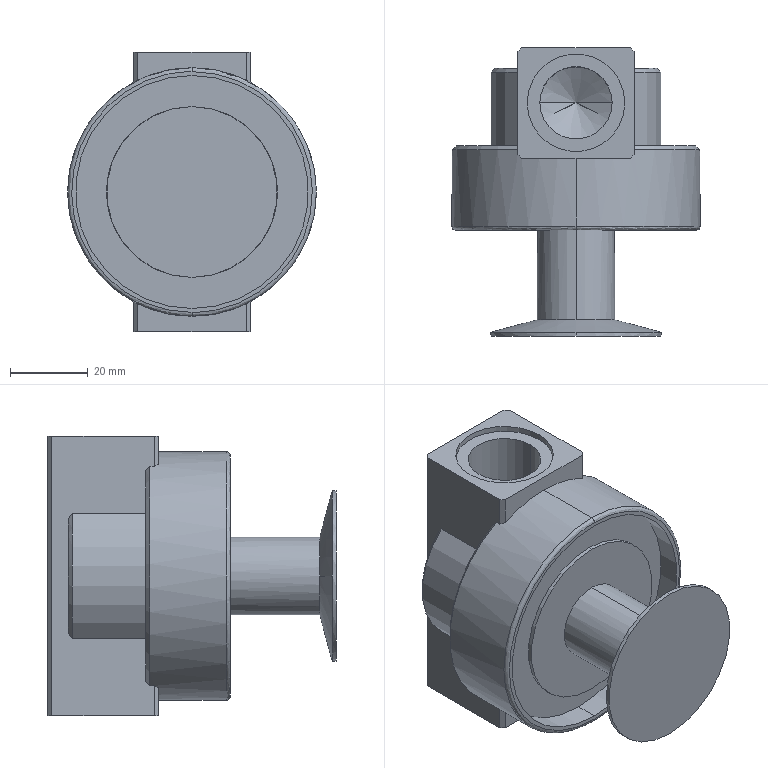Part | STEP file | _BF4000 Sw | 1 solid | 59 faces | box 64 x 74.25 x 72 mm | volume 119658 mm3 | plane 23 | cylinder 22 | cone 12 | spline 2 | commonest cylinder face diameters 44 x6 18.631 x4 20 x4 25.146 x4 60 x2 64 x2